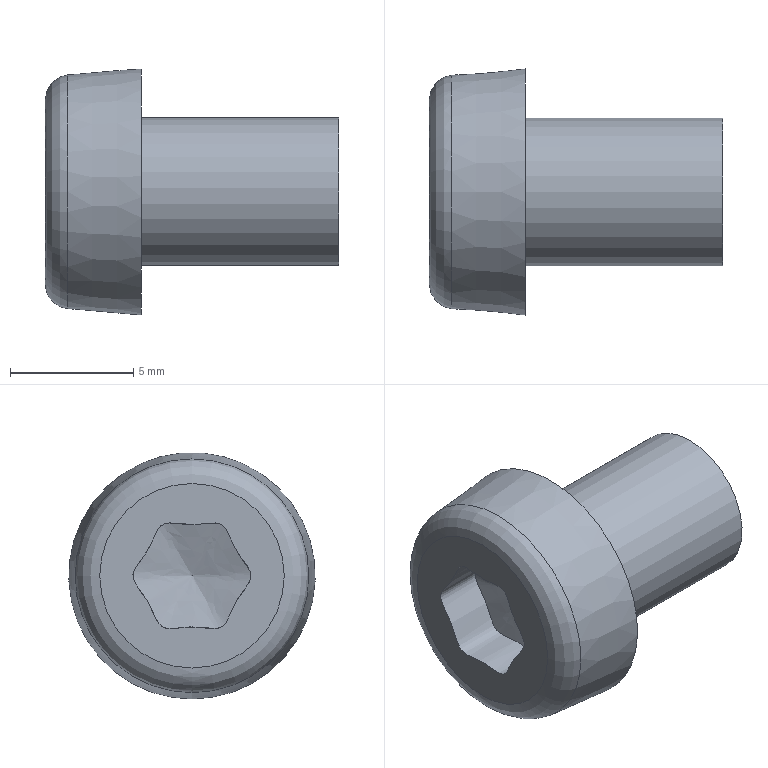Part | STEP file | hex lobular socket head cap screws-4.8 gb_GB_HEXAGON_TYPE21 M6X8-8-N | 1 solid | 8 faces | box 11.9 x 10 x 10 mm | volume 475.403 mm3 | plane 3 | spline 2 | cone 1 | cylinder 1 | torus 1 | commonest cylinder face diameters 6 x1
STEP:
#1=CARTESIAN_POINT('',(0.,0.,0.));
#2=DIRECTION('',(0.,0.,1.));
#3=DIRECTION('',(1.,0.,0.));
#4=AXIS2_PLACEMENT_3D('',#1,#2,#3);
#5=CARTESIAN_POINT('',(0.,0.,-3.742));
#6=VERTEX_POINT('',#5);
#7=CARTESIAN_POINT('',(0.,0.,0.));
#8=DIRECTION('',(-1.,0.,0.));
#9=DIRECTION('',(0.,0.,-1.));
#10=AXIS2_PLACEMENT_3D('',#7,#8,#9);
#11=CIRCLE('',#10,3.742);
#12=CARTESIAN_POINT('',(0.,0.,0.));
#13=DIRECTION('',(1.,0.,0.));
#14=DIRECTION('',(0.,0.,-1.));
#15=AXIS2_PLACEMENT_3D('',#12,#13,#14);
#16=PLANE('',#15);
#17=CARTESIAN_POINT('',(3.742,0.));
#18=CARTESIAN_POINT('',(3.742,-6.482));
#19=CARTESIAN_POINT('',(-1.871,-3.241));
#20=CARTESIAN_POINT('',(-7.485,0.));
#21=CARTESIAN_POINT('',(-1.871,3.241));
#22=CARTESIAN_POINT('',(3.742,6.482));
#23=CARTESIAN_POINT('',(3.742,0.));
#24=(BOUNDED_CURVE()B_SPLINE_CURVE(2,(#17,#18,#19,#20,#21,#22,#23),.UNSPECIFIED.,.T.,.F.)B_SPLINE_CURVE_WITH_KNOTS((1,2,2,2,2,1),(-2.094,0.,2.094,4.189,6.283,8.378),.UNSPECIFIED.)CURVE()GEOMETRIC_REPRESENTATION_ITEM()RATIONAL_B_SPLINE_CURVE((1.,0.5,1.,0.5,1.,0.5,1.))REPRESENTATION_ITEM(''));
#25=(GEOMETRIC_REPRESENTATION_CONTEXT(2)PARAMETRIC_REPRESENTATION_CONTEXT()REPRESENTATION_CONTEXT('',''));
#26=DEFINITIONAL_REPRESENTATION('',(#24),#25);
#27=PCURVE('',#16,#26);
#28=CARTESIAN_POINT('',(1.,0.,0.));
#29=DIRECTION('',(1.,0.,0.));
#30=DIRECTION('',(0.,0.,-1.));
#31=AXIS2_PLACEMENT_3D('',#28,#29,#30);
#32=TOROIDAL_SURFACE('',#31,3.742,1.);
#33=CARTESIAN_POINT('',(6.283,4.712));
#34=DIRECTION('',(-1.,0.));
#35=VECTOR('',#34,1.);
#36=LINE('',#33,#35);
#37=(GEOMETRIC_REPRESENTATION_CONTEXT(2)PARAMETRIC_REPRESENTATION_CONTEXT()REPRESENTATION_CONTEXT('',''));
#38=DEFINITIONAL_REPRESENTATION('',(#36),#37);
#39=PCURVE('',#32,#38);
#40=SURFACE_CURVE('',#11,(#27,#39),.PCURVE_S1.);
#41=EDGE_CURVE('',#6,#6,#40,.T.);
#42=ORIENTED_EDGE('',*,*,#41,.T.);
#43=EDGE_LOOP('',(#42));
#44=FACE_BOUND('',#43,.T.);
#45=CARTESIAN_POINT('',(0.,1.797,-1.038));
#46=VERTEX_POINT('',#45);
#47=CARTESIAN_POINT('',(0.,1.797,-1.038));
#48=CARTESIAN_POINT('',(0.,2.027,-0.6385));
#49=CARTESIAN_POINT('',(0.,2.765,0.));
#50=CARTESIAN_POINT('',(0.,1.659,0.9577));
#51=CARTESIAN_POINT('',(0.,1.382,2.394));
#52=CARTESIAN_POINT('',(0.,0.,1.915));
#53=CARTESIAN_POINT('',(0.,-1.382,2.394));
#54=CARTESIAN_POINT('',(0.,-1.659,0.9577));
#55=CARTESIAN_POINT('',(0.,-2.765,0.));
#56=CARTESIAN_POINT('',(0.,-1.659,-0.9577));
#57=CARTESIAN_POINT('',(0.,-1.382,-2.394));
#58=CARTESIAN_POINT('',(0.,0.,-1.915));
#59=CARTESIAN_POINT('',(0.,1.382,-2.394));
#60=CARTESIAN_POINT('',(0.,1.567,-1.437));
#61=CARTESIAN_POINT('',(0.,1.797,-1.038));
#62=B_SPLINE_CURVE_WITH_KNOTS('',3,(#47,#48,#49,#50,#51,#52,#53,#54,#55,#56,#57,#58,#59,#60,#61),.UNSPECIFIED.,.T.,.F.,(1,3,1,1,1,1,1,1,1,1,1,1,1,3,1),(-0.08333,0.,0.08333,0.1667,0.25,0.3333,0.4167,0.5,0.5833,0.6667,0.75,0.8333,0.9167,1.,1.083),.UNSPECIFIED.);
#63=CARTESIAN_POINT('',(1.038,1.797));
#64=CARTESIAN_POINT('',(0.6385,2.027));
#65=CARTESIAN_POINT('',(0.,2.765));
#66=CARTESIAN_POINT('',(-0.9577,1.659));
#67=CARTESIAN_POINT('',(-2.394,1.382));
#68=CARTESIAN_POINT('',(-1.915,0.));
#69=CARTESIAN_POINT('',(-2.394,-1.382));
#70=CARTESIAN_POINT('',(-0.9577,-1.659));
#71=CARTESIAN_POINT('',(0.,-2.765));
#72=CARTESIAN_POINT('',(0.9577,-1.659));
#73=CARTESIAN_POINT('',(2.394,-1.382));
#74=CARTESIAN_POINT('',(1.915,0.));
#75=CARTESIAN_POINT('',(2.394,1.382));
#76=CARTESIAN_POINT('',(1.437,1.567));
#77=CARTESIAN_POINT('',(1.038,1.797));
#78=B_SPLINE_CURVE_WITH_KNOTS('',3,(#63,#64,#65,#66,#67,#68,#69,#70,#71,#72,#73,#74,#75,#76,#77),.UNSPECIFIED.,.T.,.F.,(1,3,1,1,1,1,1,1,1,1,1,1,1,3,1),(-0.08333,0.,0.08333,0.1667,0.25,0.3333,0.4167,0.5,0.5833,0.6667,0.75,0.8333,0.9167,1.,1.083),.UNSPECIFIED.);
#79=(GEOMETRIC_REPRESENTATION_CONTEXT(2)PARAMETRIC_REPRESENTATION_CONTEXT()REPRESENTATION_CONTEXT('',''));
#80=DEFINITIONAL_REPRESENTATION('',(#78),#79);
#81=PCURVE('',#16,#80);
#82=CARTESIAN_POINT('',(2.,1.797,-1.038));
#83=CARTESIAN_POINT('',(0.,1.797,-1.038));
#84=CARTESIAN_POINT('',(2.,2.027,-0.6385));
#85=CARTESIAN_POINT('',(0.,2.027,-0.6385));
#86=CARTESIAN_POINT('',(2.,2.765,0.));
#87=CARTESIAN_POINT('',(0.,2.765,0.));
#88=CARTESIAN_POINT('',(2.,1.659,0.9577));
#89=CARTESIAN_POINT('',(0.,1.659,0.9577));
#90=CARTESIAN_POINT('',(2.,1.382,2.394));
#91=CARTESIAN_POINT('',(0.,1.382,2.394));
#92=CARTESIAN_POINT('',(2.,0.,1.915));
#93=CARTESIAN_POINT('',(0.,0.,1.915));
#94=CARTESIAN_POINT('',(2.,-1.382,2.394));
#95=CARTESIAN_POINT('',(0.,-1.382,2.394));
#96=CARTESIAN_POINT('',(2.,-1.659,0.9577));
#97=CARTESIAN_POINT('',(0.,-1.659,0.9577));
#98=CARTESIAN_POINT('',(2.,-2.765,0.));
#99=CARTESIAN_POINT('',(0.,-2.765,0.));
#100=CARTESIAN_POINT('',(2.,-1.659,-0.9577));
#101=CARTESIAN_POINT('',(0.,-1.659,-0.9577));
#102=CARTESIAN_POINT('',(2.,-1.382,-2.394));
#103=CARTESIAN_POINT('',(0.,-1.382,-2.394));
#104=CARTESIAN_POINT('',(2.,0.,-1.915));
#105=CARTESIAN_POINT('',(0.,0.,-1.915));
#106=CARTESIAN_POINT('',(2.,1.382,-2.394));
#107=CARTESIAN_POINT('',(0.,1.382,-2.394));
#108=CARTESIAN_POINT('',(2.,1.567,-1.437));
#109=CARTESIAN_POINT('',(0.,1.567,-1.437));
#110=CARTESIAN_POINT('',(2.,1.797,-1.038));
#111=CARTESIAN_POINT('',(0.,1.797,-1.038));
#112=B_SPLINE_SURFACE_WITH_KNOTS('',3,1,((#82,#83),(#84,#85),(#86,#87),(#88,#89),(#90,#91),(#92,#93),(#94,#95),(#96,#97),(#98,#99),(#100,#101),(#102,#103),(#104,#105),(#106,#107),(#108,#109),(#110,#111)),.UNSPECIFIED.,.T.,.F.,.F.,(1,3,1,1,1,1,1,1,1,1,1,1,1,3,1),(2,2),(-0.08333,0.,0.08333,0.1667,0.25,0.3333,0.4167,0.5,0.5833,0.6667,0.75,0.8333,0.9167,1.,1.083),(0.,1.),.UNSPECIFIED.);
#113=CARTESIAN_POINT('',(0.,1.));
#114=DIRECTION('',(1.,0.));
#115=VECTOR('',#114,1.);
#116=LINE('',#113,#115);
#117=(GEOMETRIC_REPRESENTATION_CONTEXT(2)PARAMETRIC_REPRESENTATION_CONTEXT()REPRESENTATION_CONTEXT('',''));
#118=DEFINITIONAL_REPRESENTATION('',(#116),#117);
#119=PCURVE('',#112,#118);
#120=SURFACE_CURVE('',#62,(#81,#119),.PCURVE_S1.);
#121=EDGE_CURVE('',#46,#46,#120,.T.);
#122=ORIENTED_EDGE('',*,*,#121,.T.);
#123=EDGE_LOOP('',(#122));
#124=FACE_BOUND('',#123,.T.);
#125=ADVANCED_FACE('',(#44,#124),#16,.F.);
#126=CARTESIAN_POINT('',(3.9,0.,-5.));
#127=VERTEX_POINT('',#126);
#128=CARTESIAN_POINT('',(3.9,0.,0.));
#129=DIRECTION('',(1.,0.,0.));
#130=DIRECTION('',(0.,0.,-1.));
#131=AXIS2_PLACEMENT_3D('',#128,#129,#130);
#132=CIRCLE('',#131,5.);
#133=CARTESIAN_POINT('',(3.9,0.,0.));
#134=DIRECTION('',(1.,0.,0.));
#135=DIRECTION('',(0.,0.,-1.));
#136=AXIS2_PLACEMENT_3D('',#133,#134,#135);
#137=PLANE('',#136);
#138=CARTESIAN_POINT('',(0.,0.));
#139=DIRECTION('',(1.,0.));
#140=AXIS2_PLACEMENT_2D('',#138,#139);
#141=CIRCLE('',#140,5.);
#142=(GEOMETRIC_REPRESENTATION_CONTEXT(2)PARAMETRIC_REPRESENTATION_CONTEXT()REPRESENTATION_CONTEXT('',''));
#143=DEFINITIONAL_REPRESENTATION('',(#141),#142);
#144=PCURVE('',#137,#143);
#145=CARTESIAN_POINT('',(3.9,0.,0.));
#146=DIRECTION('',(1.,0.,0.));
#147=DIRECTION('',(0.,0.,-1.));
#148=AXIS2_PLACEMENT_3D('',#145,#146,#147);
#149=CONICAL_SURFACE('',#148,5.,0.08727);
#150=CARTESIAN_POINT('',(0.,0.));
#151=DIRECTION('',(1.,0.));
#152=VECTOR('',#151,1.);
#153=LINE('',#150,#152);
#154=(GEOMETRIC_REPRESENTATION_CONTEXT(2)PARAMETRIC_REPRESENTATION_CONTEXT()REPRESENTATION_CONTEXT('',''));
#155=DEFINITIONAL_REPRESENTATION('',(#153),#154);
#156=PCURVE('',#149,#155);
#157=SURFACE_CURVE('',#132,(#144,#156),.PCURVE_S1.);
#158=EDGE_CURVE('',#127,#127,#157,.T.);
#159=ORIENTED_EDGE('',*,*,#158,.T.);
#160=EDGE_LOOP('',(#159));
#161=FACE_BOUND('',#160,.T.);
#162=CARTESIAN_POINT('',(3.9,0.,3.));
#163=VERTEX_POINT('',#162);
#164=CARTESIAN_POINT('',(3.9,0.,0.));
#165=DIRECTION('',(-1.,0.,0.));
#166=DIRECTION('',(0.,0.,1.));
#167=AXIS2_PLACEMENT_3D('',#164,#165,#166);
#168=CIRCLE('',#167,3.);
#169=CARTESIAN_POINT('',(-3.,0.));
#170=CARTESIAN_POINT('',(-3.,5.196));
#171=CARTESIAN_POINT('',(1.5,2.598));
#172=CARTESIAN_POINT('',(6.,0.));
#173=CARTESIAN_POINT('',(1.5,-2.598));
#174=CARTESIAN_POINT('',(-3.,-5.196));
#175=CARTESIAN_POINT('',(-3.,0.));
#176=(BOUNDED_CURVE()B_SPLINE_CURVE(2,(#169,#170,#171,#172,#173,#174,#175),.UNSPECIFIED.,.T.,.F.)B_SPLINE_CURVE_WITH_KNOTS((1,2,2,2,2,1),(-2.094,0.,2.094,4.189,6.283,8.378),.UNSPECIFIED.)CURVE()GEOMETRIC_REPRESENTATION_ITEM()RATIONAL_B_SPLINE_CURVE((1.,0.5,1.,0.5,1.,0.5,1.))REPRESENTATION_ITEM(''));
#177=(GEOMETRIC_REPRESENTATION_CONTEXT(2)PARAMETRIC_REPRESENTATION_CONTEXT()REPRESENTATION_CONTEXT('',''));
#178=DEFINITIONAL_REPRESENTATION('',(#176),#177);
#179=PCURVE('',#137,#178);
#180=CARTESIAN_POINT('',(0.,0.,0.));
#181=DIRECTION('',(-1.,0.,0.));
#182=DIRECTION('',(0.,0.,1.));
#183=AXIS2_PLACEMENT_3D('',#180,#181,#182);
#184=CYLINDRICAL_SURFACE('',#183,3.);
#185=CARTESIAN_POINT('',(0.,-3.9));
#186=DIRECTION('',(1.,0.));
#187=VECTOR('',#186,1.);
#188=LINE('',#185,#187);
#189=(GEOMETRIC_REPRESENTATION_CONTEXT(2)PARAMETRIC_REPRESENTATION_CONTEXT()REPRESENTATION_CONTEXT('',''));
#190=DEFINITIONAL_REPRESENTATION('',(#188),#189);
#191=PCURVE('',#184,#190);
#192=SURFACE_CURVE('',#168,(#179,#191),.PCURVE_S1.);
#193=EDGE_CURVE('',#163,#163,#192,.T.);
#194=ORIENTED_EDGE('',*,*,#193,.T.);
#195=EDGE_LOOP('',(#194));
#196=FACE_BOUND('',#195,.T.);
#197=ADVANCED_FACE('',(#161,#196),#137,.T.);
#198=CARTESIAN_POINT('',(0.9128,0.,-4.739));
#199=VERTEX_POINT('',#198);
#200=CARTESIAN_POINT('',(0.9128,0.,0.));
#201=DIRECTION('',(1.,0.,0.));
#202=DIRECTION('',(0.,0.,-1.));
#203=AXIS2_PLACEMENT_3D('',#200,#201,#202);
#204=CIRCLE('',#203,4.739);
#205=CARTESIAN_POINT('',(0.,-2.987));
#206=DIRECTION('',(1.,0.));
#207=VECTOR('',#206,1.);
#208=LINE('',#205,#207);
#209=(GEOMETRIC_REPRESENTATION_CONTEXT(2)PARAMETRIC_REPRESENTATION_CONTEXT()REPRESENTATION_CONTEXT('',''));
#210=DEFINITIONAL_REPRESENTATION('',(#208),#209);
#211=PCURVE('',#149,#210);
#212=CARTESIAN_POINT('',(0.,6.196));
#213=DIRECTION('',(1.,0.));
#214=VECTOR('',#213,1.);
#215=LINE('',#212,#214);
#216=(GEOMETRIC_REPRESENTATION_CONTEXT(2)PARAMETRIC_REPRESENTATION_CONTEXT()REPRESENTATION_CONTEXT('',''));
#217=DEFINITIONAL_REPRESENTATION('',(#215),#216);
#218=PCURVE('',#32,#217);
#219=SURFACE_CURVE('',#204,(#211,#218),.PCURVE_S1.);
#220=EDGE_CURVE('',#199,#199,#219,.T.);
#221=ORIENTED_EDGE('',*,*,#220,.T.);
#222=CARTESIAN_POINT('',(0.9128,0.,-4.739));
#223=CARTESIAN_POINT('',(3.9,0.,-5.));
#224=B_SPLINE_CURVE_WITH_KNOTS('',1,(#222,#223),.UNSPECIFIED.,.F.,.F.,(2,2),(-2.999,0.),.PIECEWISE_BEZIER_KNOTS.);
#225=CARTESIAN_POINT('',(6.283,0.));
#226=DIRECTION('',(0.,1.));
#227=VECTOR('',#226,1.);
#228=LINE('',#225,#227);
#229=(GEOMETRIC_REPRESENTATION_CONTEXT(2)PARAMETRIC_REPRESENTATION_CONTEXT()REPRESENTATION_CONTEXT('',''));
#230=DEFINITIONAL_REPRESENTATION('',(#228),#229);
#231=PCURVE('',#149,#230);
#232=CARTESIAN_POINT('',(0.,0.));
#233=DIRECTION('',(0.,1.));
#234=VECTOR('',#233,1.);
#235=LINE('',#232,#234);
#236=(GEOMETRIC_REPRESENTATION_CONTEXT(2)PARAMETRIC_REPRESENTATION_CONTEXT()REPRESENTATION_CONTEXT('',''));
#237=DEFINITIONAL_REPRESENTATION('',(#235),#236);
#238=PCURVE('',#149,#237);
#239=SEAM_CURVE('',#224,(#231,#238),.PCURVE_S1.);
#240=EDGE_CURVE('',#199,#127,#239,.T.);
#241=ORIENTED_EDGE('',*,*,#240,.T.);
#242=ORIENTED_EDGE('',*,*,#158,.F.);
#243=ORIENTED_EDGE('',*,*,#240,.F.);
#244=EDGE_LOOP('',(#221,#241,#242,#243));
#245=FACE_BOUND('',#244,.T.);
#246=ADVANCED_FACE('',(#245),#149,.T.);
#247=CARTESIAN_POINT('',(11.9,0.,3.));
#248=VERTEX_POINT('',#247);
#249=CARTESIAN_POINT('',(11.9,0.,0.));
#250=DIRECTION('',(-1.,0.,0.));
#251=DIRECTION('',(0.,0.,1.));
#252=AXIS2_PLACEMENT_3D('',#249,#250,#251);
#253=CIRCLE('',#252,3.);
#254=CARTESIAN_POINT('',(11.9,3.,0.));
#255=DIRECTION('',(-1.,0.,0.));
#256=DIRECTION('',(0.,0.,1.));
#257=AXIS2_PLACEMENT_3D('',#254,#255,#256);
#258=PLANE('',#257);
#259=CARTESIAN_POINT('',(0.,-3.));
#260=DIRECTION('',(1.,0.));
#261=AXIS2_PLACEMENT_2D('',#259,#260);
#262=CIRCLE('',#261,3.);
#263=(GEOMETRIC_REPRESENTATION_CONTEXT(2)PARAMETRIC_REPRESENTATION_CONTEXT()REPRESENTATION_CONTEXT('',''));
#264=DEFINITIONAL_REPRESENTATION('',(#262),#263);
#265=PCURVE('',#258,#264);
#266=CARTESIAN_POINT('',(0.,-11.9));
#267=DIRECTION('',(1.,0.));
#268=VECTOR('',#267,1.);
#269=LINE('',#266,#268);
#270=(GEOMETRIC_REPRESENTATION_CONTEXT(2)PARAMETRIC_REPRESENTATION_CONTEXT()REPRESENTATION_CONTEXT('',''));
#271=DEFINITIONAL_REPRESENTATION('',(#269),#270);
#272=PCURVE('',#184,#271);
#273=SURFACE_CURVE('',#253,(#265,#272),.PCURVE_S1.);
#274=EDGE_CURVE('',#248,#248,#273,.T.);
#275=ORIENTED_EDGE('',*,*,#274,.F.);
#276=EDGE_LOOP('',(#275));
#277=FACE_BOUND('',#276,.T.);
#278=ADVANCED_FACE('',(#277),#258,.F.);
#279=ORIENTED_EDGE('',*,*,#193,.F.);
#280=CARTESIAN_POINT('',(11.9,0.,3.));
#281=CARTESIAN_POINT('',(3.9,0.,3.));
#282=B_SPLINE_CURVE_WITH_KNOTS('',1,(#280,#281),.UNSPECIFIED.,.F.,.F.,(2,2),(-11.9,-3.9),.PIECEWISE_BEZIER_KNOTS.);
#283=CARTESIAN_POINT('',(0.,0.));
#284=DIRECTION('',(0.,1.));
#285=VECTOR('',#284,1.);
#286=LINE('',#283,#285);
#287=(GEOMETRIC_REPRESENTATION_CONTEXT(2)PARAMETRIC_REPRESENTATION_CONTEXT()REPRESENTATION_CONTEXT('',''));
#288=DEFINITIONAL_REPRESENTATION('',(#286),#287);
#289=PCURVE('',#184,#288);
#290=CARTESIAN_POINT('',(6.283,0.));
#291=DIRECTION('',(0.,1.));
#292=VECTOR('',#291,1.);
#293=LINE('',#290,#292);
#294=(GEOMETRIC_REPRESENTATION_CONTEXT(2)PARAMETRIC_REPRESENTATION_CONTEXT()REPRESENTATION_CONTEXT('',''));
#295=DEFINITIONAL_REPRESENTATION('',(#293),#294);
#296=PCURVE('',#184,#295);
#297=SEAM_CURVE('',#282,(#289,#296),.PCURVE_S1.);
#298=EDGE_CURVE('',#248,#163,#297,.T.);
#299=ORIENTED_EDGE('',*,*,#298,.F.);
#300=ORIENTED_EDGE('',*,*,#274,.T.);
#301=ORIENTED_EDGE('',*,*,#298,.T.);
#302=EDGE_LOOP('',(#279,#299,#300,#301));
#303=FACE_BOUND('',#302,.T.);
#304=ADVANCED_FACE('',(#303),#184,.T.);
#305=CARTESIAN_POINT('',(2.,1.797,-1.038));
#306=VERTEX_POINT('',#305);
#307=CARTESIAN_POINT('',(2.,1.797,-1.038));
#308=CARTESIAN_POINT('',(2.,1.567,-1.437));
#309=CARTESIAN_POINT('',(2.,1.382,-2.394));
#310=CARTESIAN_POINT('',(2.,0.,-1.915));
#311=CARTESIAN_POINT('',(2.,-1.382,-2.394));
#312=CARTESIAN_POINT('',(2.,-1.659,-0.9577));
#313=CARTESIAN_POINT('',(2.,-2.765,0.));
#314=CARTESIAN_POINT('',(2.,-1.659,0.9577));
#315=CARTESIAN_POINT('',(2.,-1.382,2.394));
#316=CARTESIAN_POINT('',(2.,0.,1.915));
#317=CARTESIAN_POINT('',(2.,1.382,2.394));
#318=CARTESIAN_POINT('',(2.,1.659,0.9577));
#319=CARTESIAN_POINT('',(2.,2.765,0.));
#320=CARTESIAN_POINT('',(2.,2.027,-0.6385));
#321=CARTESIAN_POINT('',(2.,1.797,-1.038));
#322=B_SPLINE_CURVE_WITH_KNOTS('',3,(#307,#308,#309,#310,#311,#312,#313,#314,#315,#316,#317,#318,#319,#320,#321),.UNSPECIFIED.,.T.,.F.,(1,3,1,1,1,1,1,1,1,1,1,1,1,3,1),(-0.08333,0.,0.08333,0.1667,0.25,0.3333,0.4167,0.5,0.5833,0.6667,0.75,0.8333,0.9167,1.,1.083),.UNSPECIFIED.);
#323=CARTESIAN_POINT('',(1.,0.));
#324=DIRECTION('',(-1.,0.));
#325=VECTOR('',#324,1.);
#326=LINE('',#323,#325);
#327=(GEOMETRIC_REPRESENTATION_CONTEXT(2)PARAMETRIC_REPRESENTATION_CONTEXT()REPRESENTATION_CONTEXT('',''));
#328=DEFINITIONAL_REPRESENTATION('',(#326),#327);
#329=PCURVE('',#112,#328);
#330=CARTESIAN_POINT('',(2.667,0.,0.));
#331=CARTESIAN_POINT('',(2.,1.797,-1.038));
#332=CARTESIAN_POINT('',(2.667,0.,0.));
#333=CARTESIAN_POINT('',(2.,1.567,-1.437));
#334=CARTESIAN_POINT('',(2.667,0.,0.));
#335=CARTESIAN_POINT('',(2.,1.382,-2.394));
#336=CARTESIAN_POINT('',(2.667,0.,0.));
#337=CARTESIAN_POINT('',(2.,0.,-1.915));
#338=CARTESIAN_POINT('',(2.667,0.,0.));
#339=CARTESIAN_POINT('',(2.,-1.382,-2.394));
#340=CARTESIAN_POINT('',(2.667,0.,0.));
#341=CARTESIAN_POINT('',(2.,-1.659,-0.9577));
#342=CARTESIAN_POINT('',(2.667,0.,0.));
#343=CARTESIAN_POINT('',(2.,-2.765,0.));
#344=CARTESIAN_POINT('',(2.667,0.,0.));
#345=CARTESIAN_POINT('',(2.,-1.659,0.9577));
#346=CARTESIAN_POINT('',(2.667,0.,0.));
#347=CARTESIAN_POINT('',(2.,-1.382,2.394));
#348=CARTESIAN_POINT('',(2.667,0.,0.));
#349=CARTESIAN_POINT('',(2.,0.,1.915));
#350=CARTESIAN_POINT('',(2.667,0.,0.));
#351=CARTESIAN_POINT('',(2.,1.382,2.394));
#352=CARTESIAN_POINT('',(2.667,0.,0.));
#353=CARTESIAN_POINT('',(2.,1.659,0.9577));
#354=CARTESIAN_POINT('',(2.667,0.,0.));
#355=CARTESIAN_POINT('',(2.,2.765,0.));
#356=CARTESIAN_POINT('',(2.667,0.,0.));
#357=CARTESIAN_POINT('',(2.,2.027,-0.6385));
#358=CARTESIAN_POINT('',(2.667,0.,0.));
#359=CARTESIAN_POINT('',(2.,1.797,-1.038));
#360=B_SPLINE_SURFACE_WITH_KNOTS('',3,1,((#330,#331),(#332,#333),(#334,#335),(#336,#337),(#338,#339),(#340,#341),(#342,#343),(#344,#345),(#346,#347),(#348,#349),(#350,#351),(#352,#353),(#354,#355),(#356,#357),(#358,#359)),.UNSPECIFIED.,.T.,.F.,.F.,(1,3,1,1,1,1,1,1,1,1,1,1,1,3,1),(2,2),(-0.08333,0.,0.08333,0.1667,0.25,0.3333,0.4167,0.5,0.5833,0.6667,0.75,0.8333,0.9167,1.,1.083),(0.,1.),.UNSPECIFIED.);
#361=CARTESIAN_POINT('',(0.,1.));
#362=DIRECTION('',(1.,0.));
#363=VECTOR('',#362,1.);
#364=LINE('',#361,#363);
#365=(GEOMETRIC_REPRESENTATION_CONTEXT(2)PARAMETRIC_REPRESENTATION_CONTEXT()REPRESENTATION_CONTEXT('',''));
#366=DEFINITIONAL_REPRESENTATION('',(#364),#365);
#367=PCURVE('',#360,#366);
#368=SURFACE_CURVE('',#322,(#329,#367),.PCURVE_S1.);
#369=EDGE_CURVE('',#306,#306,#368,.T.);
#370=ORIENTED_EDGE('',*,*,#369,.F.);
#371=CARTESIAN_POINT('',(2.,1.797,-1.038));
#372=CARTESIAN_POINT('',(0.,1.797,-1.038));
#373=B_SPLINE_CURVE_WITH_KNOTS('',1,(#371,#372),.UNSPECIFIED.,.F.,.F.,(2,2),(0.,1.),.PIECEWISE_BEZIER_KNOTS.);
#374=CARTESIAN_POINT('',(1.,0.));
#375=DIRECTION('',(0.,1.));
#376=VECTOR('',#375,1.);
#377=LINE('',#374,#376);
#378=(GEOMETRIC_REPRESENTATION_CONTEXT(2)PARAMETRIC_REPRESENTATION_CONTEXT()REPRESENTATION_CONTEXT('',''));
#379=DEFINITIONAL_REPRESENTATION('',(#377),#378);
#380=PCURVE('',#112,#379);
#381=CARTESIAN_POINT('',(0.,0.));
#382=DIRECTION('',(0.,1.));
#383=VECTOR('',#382,1.);
#384=LINE('',#381,#383);
#385=(GEOMETRIC_REPRESENTATION_CONTEXT(2)PARAMETRIC_REPRESENTATION_CONTEXT()REPRESENTATION_CONTEXT('',''));
#386=DEFINITIONAL_REPRESENTATION('',(#384),#385);
#387=PCURVE('',#112,#386);
#388=SEAM_CURVE('',#373,(#380,#387),.PCURVE_S1.);
#389=EDGE_CURVE('',#306,#46,#388,.T.);
#390=ORIENTED_EDGE('',*,*,#389,.T.);
#391=ORIENTED_EDGE('',*,*,#121,.F.);
#392=ORIENTED_EDGE('',*,*,#389,.F.);
#393=EDGE_LOOP('',(#370,#390,#391,#392));
#394=FACE_BOUND('',#393,.T.);
#395=ADVANCED_FACE('',(#394),#112,.T.);
#396=ORIENTED_EDGE('',*,*,#369,.F.);
#397=CARTESIAN_POINT('',(2.667,0.,0.));
#398=VERTEX_POINT('',#397);
#399=CARTESIAN_POINT('',(2.667,0.,0.));
#400=CARTESIAN_POINT('',(2.,1.797,-1.038));
#401=B_SPLINE_CURVE_WITH_KNOTS('',1,(#399,#400),.UNSPECIFIED.,.F.,.F.,(2,2),(0.,1.),.PIECEWISE_BEZIER_KNOTS.);
#402=CARTESIAN_POINT('',(0.,0.));
#403=DIRECTION('',(0.,1.));
#404=VECTOR('',#403,1.);
#405=LINE('',#402,#404);
#406=(GEOMETRIC_REPRESENTATION_CONTEXT(2)PARAMETRIC_REPRESENTATION_CONTEXT()REPRESENTATION_CONTEXT('',''));
#407=DEFINITIONAL_REPRESENTATION('',(#405),#406);
#408=PCURVE('',#360,#407);
#409=CARTESIAN_POINT('',(1.,0.));
#410=DIRECTION('',(0.,1.));
#411=VECTOR('',#410,1.);
#412=LINE('',#409,#411);
#413=(GEOMETRIC_REPRESENTATION_CONTEXT(2)PARAMETRIC_REPRESENTATION_CONTEXT()REPRESENTATION_CONTEXT('',''));
#414=DEFINITIONAL_REPRESENTATION('',(#412),#413);
#415=PCURVE('',#360,#414);
#416=SEAM_CURVE('',#401,(#408,#415),.PCURVE_S1.);
#417=EDGE_CURVE('',#398,#306,#416,.T.);
#418=ORIENTED_EDGE('',*,*,#417,.F.);
#419=ORIENTED_EDGE('',*,*,#417,.T.);
#420=EDGE_LOOP('',(#396,#418,#419));
#421=FACE_BOUND('',#420,.F.);
#422=ADVANCED_FACE('',(#421),#360,.F.);
#423=ORIENTED_EDGE('',*,*,#41,.F.);
#424=CARTESIAN_POINT('',(0.,0.,-3.742));
#425=CARTESIAN_POINT('',(0.,0.,-3.994));
#426=CARTESIAN_POINT('',(0.07555,0.,-4.24));
#427=CARTESIAN_POINT('',(0.2212,0.,-4.456));
#428=CARTESIAN_POINT('',(0.4233,0.,-4.62));
#429=CARTESIAN_POINT('',(0.6619,0.,-4.717));
#430=CARTESIAN_POINT('',(0.9128,0.,-4.739));
#431=(BOUNDED_CURVE()B_SPLINE_CURVE(6,(#424,#425,#426,#427,#428,#429,#430),.UNSPECIFIED.,.F.,.F.)B_SPLINE_CURVE_WITH_KNOTS((7,7),(4.712,6.196),.PIECEWISE_BEZIER_KNOTS.)CURVE()GEOMETRIC_REPRESENTATION_ITEM()RATIONAL_B_SPLINE_CURVE((1.028,1.009,0.9981,0.9946,0.9981,1.009,1.028))REPRESENTATION_ITEM(''));
#432=CARTESIAN_POINT('',(6.283,0.));
#433=DIRECTION('',(0.,1.));
#434=VECTOR('',#433,1.);
#435=LINE('',#432,#434);
#436=(GEOMETRIC_REPRESENTATION_CONTEXT(2)PARAMETRIC_REPRESENTATION_CONTEXT()REPRESENTATION_CONTEXT('',''));
#437=DEFINITIONAL_REPRESENTATION('',(#435),#436);
#438=PCURVE('',#32,#437);
#439=CARTESIAN_POINT('',(0.,0.));
#440=DIRECTION('',(0.,1.));
#441=VECTOR('',#440,1.);
#442=LINE('',#439,#441);
#443=(GEOMETRIC_REPRESENTATION_CONTEXT(2)PARAMETRIC_REPRESENTATION_CONTEXT()REPRESENTATION_CONTEXT('',''));
#444=DEFINITIONAL_REPRESENTATION('',(#442),#443);
#445=PCURVE('',#32,#444);
#446=SEAM_CURVE('',#431,(#438,#445),.PCURVE_S1.);
#447=EDGE_CURVE('',#6,#199,#446,.T.);
#448=ORIENTED_EDGE('',*,*,#447,.T.);
#449=ORIENTED_EDGE('',*,*,#220,.F.);
#450=ORIENTED_EDGE('',*,*,#447,.F.);
#451=EDGE_LOOP('',(#423,#448,#449,#450));
#452=FACE_BOUND('',#451,.T.);
#453=ADVANCED_FACE('',(#452),#32,.T.);
#454=CLOSED_SHELL('',(#125,#197,#246,#278,#304,#395,#422,#453));
#455=MANIFOLD_SOLID_BREP('',#454);
#456=(LENGTH_UNIT()NAMED_UNIT(*)SI_UNIT(.MILLI.,.METRE.));
#457=UNCERTAINTY_MEASURE_WITH_UNIT(LENGTH_MEASURE(0.00001),#456,'','');
#458=(NAMED_UNIT(*)PLANE_ANGLE_UNIT()SI_UNIT($,.RADIAN.));
#459=(NAMED_UNIT(*)SI_UNIT($,.STERADIAN.)SOLID_ANGLE_UNIT());
#460=(GEOMETRIC_REPRESENTATION_CONTEXT(3)GLOBAL_UNCERTAINTY_ASSIGNED_CONTEXT((#457))GLOBAL_UNIT_ASSIGNED_CONTEXT((#456,#458,#459))REPRESENTATION_CONTEXT('',''));
#461=ADVANCED_BREP_SHAPE_REPRESENTATION('',(#4,#455),#460);